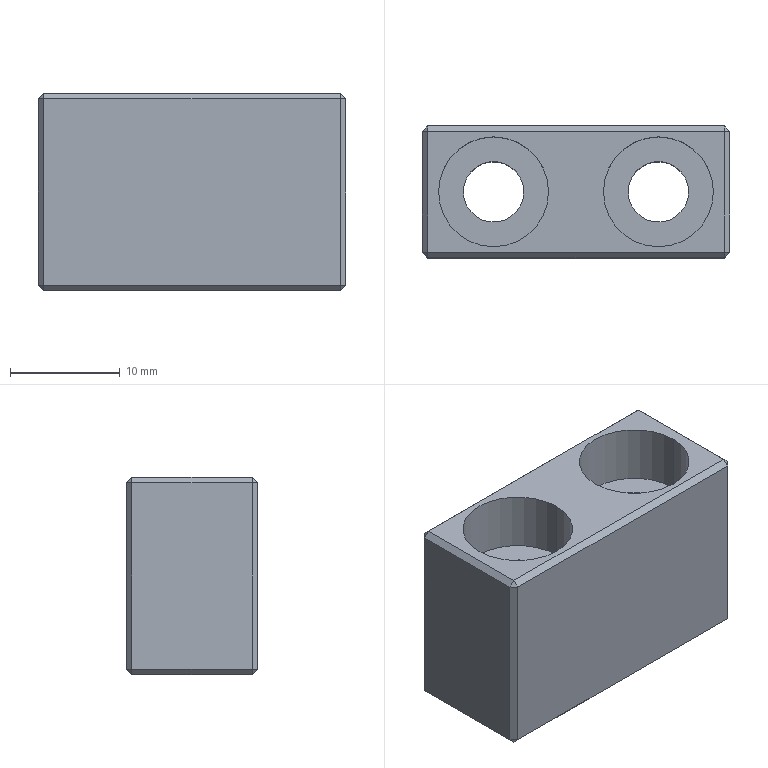Part | SolidWorks | features Chamfer 1, Extrusion 1, HoleWzd 1 | 1 solid | 36 faces | box 28 x 12 x 18 mm | volume 4573 mm3 | plane 28 | cylinder 8 | commonest cylinder face diameters 5.5 x4 10 x4
STEP:
#1=CARTESIAN_POINT('',(-12.5,6.,3.6));
#2=VERTEX_POINT('',#1);
#3=CARTESIAN_POINT('',(-2.5,6.,3.6));
#4=VERTEX_POINT('',#3);
#5=CARTESIAN_POINT('',(-7.5,6.,3.6));
#6=DIRECTION('',(0.,0.,1.));
#7=DIRECTION('',(1.,0.,0.));
#8=AXIS2_PLACEMENT_3D('',#5,#6,#7);
#9=CIRCLE('',#8,5.);
#10=EDGE_CURVE('',#2,#4,#9,.T.);
#11=ORIENTED_EDGE('',*,*,#10,.F.);
#12=CARTESIAN_POINT('',(-12.5,6.,9.));
#13=VERTEX_POINT('',#12);
#14=CARTESIAN_POINT('',(-12.5,6.,9.));
#15=DIRECTION('',(0.,0.,1.));
#16=VECTOR('',#15,1000.);
#17=LINE('',#14,#16);
#18=EDGE_CURVE('',#2,#13,#17,.T.);
#19=ORIENTED_EDGE('',*,*,#18,.T.);
#20=CARTESIAN_POINT('',(-2.5,6.,9.));
#21=VERTEX_POINT('',#20);
#22=CARTESIAN_POINT('',(-7.5,6.,9.));
#23=DIRECTION('',(0.,0.,1.));
#24=DIRECTION('',(1.,0.,0.));
#25=AXIS2_PLACEMENT_3D('',#22,#23,#24);
#26=CIRCLE('',#25,5.);
#27=EDGE_CURVE('',#13,#21,#26,.T.);
#28=ORIENTED_EDGE('',*,*,#27,.T.);
#29=CARTESIAN_POINT('',(-2.5,6.,9.));
#30=DIRECTION('',(0.,0.,1.));
#31=VECTOR('',#30,1000.);
#32=LINE('',#29,#31);
#33=EDGE_CURVE('',#4,#21,#32,.T.);
#34=ORIENTED_EDGE('',*,*,#33,.F.);
#35=EDGE_LOOP('',(#11,#19,#28,#34));
#36=FACE_OUTER_BOUND('',#35,.T.);
#37=CARTESIAN_POINT('',(-7.5,6.,9.));
#38=DIRECTION('',(0.,0.,1.));
#39=DIRECTION('',(1.,0.,0.));
#40=AXIS2_PLACEMENT_3D('',#37,#38,#39);
#41=CYLINDRICAL_SURFACE('',#40,5.);
#42=ADVANCED_FACE('',(#36),#41,.F.);
#43=CARTESIAN_POINT('',(-10.25,6.,-9.));
#44=VERTEX_POINT('',#43);
#45=CARTESIAN_POINT('',(-4.75,6.,-9.));
#46=VERTEX_POINT('',#45);
#47=CARTESIAN_POINT('',(-7.5,6.,-9.));
#48=DIRECTION('',(0.,0.,1.));
#49=DIRECTION('',(1.,0.,0.));
#50=AXIS2_PLACEMENT_3D('',#47,#48,#49);
#51=CIRCLE('',#50,2.75);
#52=EDGE_CURVE('',#44,#46,#51,.T.);
#53=ORIENTED_EDGE('',*,*,#52,.F.);
#54=CARTESIAN_POINT('',(-10.25,6.,3.6));
#55=VERTEX_POINT('',#54);
#56=CARTESIAN_POINT('',(-10.25,6.,9.));
#57=DIRECTION('',(0.,0.,1.));
#58=VECTOR('',#57,1000.);
#59=LINE('',#56,#58);
#60=EDGE_CURVE('',#44,#55,#59,.T.);
#61=ORIENTED_EDGE('',*,*,#60,.T.);
#62=CARTESIAN_POINT('',(-4.75,6.,3.6));
#63=VERTEX_POINT('',#62);
#64=CARTESIAN_POINT('',(-7.5,6.,3.6));
#65=DIRECTION('',(0.,0.,1.));
#66=DIRECTION('',(1.,0.,0.));
#67=AXIS2_PLACEMENT_3D('',#64,#65,#66);
#68=CIRCLE('',#67,2.75);
#69=EDGE_CURVE('',#55,#63,#68,.T.);
#70=ORIENTED_EDGE('',*,*,#69,.T.);
#71=CARTESIAN_POINT('',(-4.75,6.,9.));
#72=DIRECTION('',(0.,0.,1.));
#73=VECTOR('',#72,1000.);
#74=LINE('',#71,#73);
#75=EDGE_CURVE('',#46,#63,#74,.T.);
#76=ORIENTED_EDGE('',*,*,#75,.F.);
#77=EDGE_LOOP('',(#53,#61,#70,#76));
#78=FACE_OUTER_BOUND('',#77,.T.);
#79=CARTESIAN_POINT('',(-7.5,6.,9.));
#80=DIRECTION('',(0.,0.,1.));
#81=DIRECTION('',(1.,0.,0.));
#82=AXIS2_PLACEMENT_3D('',#79,#80,#81);
#83=CYLINDRICAL_SURFACE('',#82,2.75);
#84=ADVANCED_FACE('',(#78),#83,.F.);
#85=CARTESIAN_POINT('',(2.5,6.,3.6));
#86=VERTEX_POINT('',#85);
#87=CARTESIAN_POINT('',(12.5,6.,3.6));
#88=VERTEX_POINT('',#87);
#89=CARTESIAN_POINT('',(7.5,6.,3.6));
#90=DIRECTION('',(0.,0.,1.));
#91=DIRECTION('',(1.,0.,0.));
#92=AXIS2_PLACEMENT_3D('',#89,#90,#91);
#93=CIRCLE('',#92,5.);
#94=EDGE_CURVE('',#86,#88,#93,.T.);
#95=ORIENTED_EDGE('',*,*,#94,.F.);
#96=CARTESIAN_POINT('',(2.5,6.,9.));
#97=VERTEX_POINT('',#96);
#98=CARTESIAN_POINT('',(2.5,6.,9.));
#99=DIRECTION('',(0.,0.,1.));
#100=VECTOR('',#99,1000.);
#101=LINE('',#98,#100);
#102=EDGE_CURVE('',#86,#97,#101,.T.);
#103=ORIENTED_EDGE('',*,*,#102,.T.);
#104=CARTESIAN_POINT('',(12.5,6.,9.));
#105=VERTEX_POINT('',#104);
#106=CARTESIAN_POINT('',(7.5,6.,9.));
#107=DIRECTION('',(0.,0.,1.));
#108=DIRECTION('',(1.,0.,0.));
#109=AXIS2_PLACEMENT_3D('',#106,#107,#108);
#110=CIRCLE('',#109,5.);
#111=EDGE_CURVE('',#97,#105,#110,.T.);
#112=ORIENTED_EDGE('',*,*,#111,.T.);
#113=CARTESIAN_POINT('',(12.5,6.,9.));
#114=DIRECTION('',(0.,0.,1.));
#115=VECTOR('',#114,1000.);
#116=LINE('',#113,#115);
#117=EDGE_CURVE('',#88,#105,#116,.T.);
#118=ORIENTED_EDGE('',*,*,#117,.F.);
#119=EDGE_LOOP('',(#95,#103,#112,#118));
#120=FACE_OUTER_BOUND('',#119,.T.);
#121=CARTESIAN_POINT('',(7.5,6.,9.));
#122=DIRECTION('',(0.,0.,1.));
#123=DIRECTION('',(1.,0.,0.));
#124=AXIS2_PLACEMENT_3D('',#121,#122,#123);
#125=CYLINDRICAL_SURFACE('',#124,5.);
#126=ADVANCED_FACE('',(#120),#125,.F.);
#127=CARTESIAN_POINT('',(4.75,6.,-9.));
#128=VERTEX_POINT('',#127);
#129=CARTESIAN_POINT('',(10.25,6.,-9.));
#130=VERTEX_POINT('',#129);
#131=CARTESIAN_POINT('',(7.5,6.,-9.));
#132=DIRECTION('',(0.,0.,1.));
#133=DIRECTION('',(1.,0.,0.));
#134=AXIS2_PLACEMENT_3D('',#131,#132,#133);
#135=CIRCLE('',#134,2.75);
#136=EDGE_CURVE('',#128,#130,#135,.T.);
#137=ORIENTED_EDGE('',*,*,#136,.F.);
#138=CARTESIAN_POINT('',(4.75,6.,3.6));
#139=VERTEX_POINT('',#138);
#140=CARTESIAN_POINT('',(4.75,6.,9.));
#141=DIRECTION('',(0.,0.,1.));
#142=VECTOR('',#141,1000.);
#143=LINE('',#140,#142);
#144=EDGE_CURVE('',#128,#139,#143,.T.);
#145=ORIENTED_EDGE('',*,*,#144,.T.);
#146=CARTESIAN_POINT('',(10.25,6.,3.6));
#147=VERTEX_POINT('',#146);
#148=CARTESIAN_POINT('',(7.5,6.,3.6));
#149=DIRECTION('',(0.,0.,1.));
#150=DIRECTION('',(1.,0.,0.));
#151=AXIS2_PLACEMENT_3D('',#148,#149,#150);
#152=CIRCLE('',#151,2.75);
#153=EDGE_CURVE('',#139,#147,#152,.T.);
#154=ORIENTED_EDGE('',*,*,#153,.T.);
#155=CARTESIAN_POINT('',(10.25,6.,9.));
#156=DIRECTION('',(0.,0.,1.));
#157=VECTOR('',#156,1000.);
#158=LINE('',#155,#157);
#159=EDGE_CURVE('',#130,#147,#158,.T.);
#160=ORIENTED_EDGE('',*,*,#159,.F.);
#161=EDGE_LOOP('',(#137,#145,#154,#160));
#162=FACE_OUTER_BOUND('',#161,.T.);
#163=CARTESIAN_POINT('',(7.5,6.,9.));
#164=DIRECTION('',(0.,0.,1.));
#165=DIRECTION('',(1.,0.,0.));
#166=AXIS2_PLACEMENT_3D('',#163,#164,#165);
#167=CYLINDRICAL_SURFACE('',#166,2.75);
#168=ADVANCED_FACE('',(#162),#167,.F.);
#169=CARTESIAN_POINT('',(14.,11.5,-8.5));
#170=VERTEX_POINT('',#169);
#171=CARTESIAN_POINT('',(14.,11.5,8.5));
#172=VERTEX_POINT('',#171);
#173=CARTESIAN_POINT('',(14.,11.5,9.));
#174=DIRECTION('',(0.,0.,1.));
#175=VECTOR('',#174,1000.);
#176=LINE('',#173,#175);
#177=EDGE_CURVE('',#170,#172,#176,.T.);
#178=ORIENTED_EDGE('',*,*,#177,.T.);
#179=CARTESIAN_POINT('',(14.,0.5,8.5));
#180=VERTEX_POINT('',#179);
#181=CARTESIAN_POINT('',(14.,12.,8.5));
#182=DIRECTION('',(0.,-1.,0.));
#183=VECTOR('',#182,1000.);
#184=LINE('',#181,#183);
#185=EDGE_CURVE('',#172,#180,#184,.T.);
#186=ORIENTED_EDGE('',*,*,#185,.T.);
#187=CARTESIAN_POINT('',(14.,0.5,-8.5));
#188=VERTEX_POINT('',#187);
#189=CARTESIAN_POINT('',(14.,0.5,-9.));
#190=DIRECTION('',(0.,0.,-1.));
#191=VECTOR('',#190,1000.);
#192=LINE('',#189,#191);
#193=EDGE_CURVE('',#180,#188,#192,.T.);
#194=ORIENTED_EDGE('',*,*,#193,.T.);
#195=CARTESIAN_POINT('',(14.,12.,-8.5));
#196=DIRECTION('',(0.,1.,0.));
#197=VECTOR('',#196,1000.);
#198=LINE('',#195,#197);
#199=EDGE_CURVE('',#188,#170,#198,.T.);
#200=ORIENTED_EDGE('',*,*,#199,.T.);
#201=EDGE_LOOP('',(#178,#186,#194,#200));
#202=FACE_OUTER_BOUND('',#201,.T.);
#203=CARTESIAN_POINT('',(14.,12.,-9.));
#204=DIRECTION('',(-1.,0.,0.));
#205=DIRECTION('',(0.,0.,1.));
#206=AXIS2_PLACEMENT_3D('',#203,#204,#205);
#207=PLANE('',#206);
#208=ADVANCED_FACE('',(#202),#207,.F.);
#209=CARTESIAN_POINT('',(13.5,11.5,-9.));
#210=VERTEX_POINT('',#209);
#211=CARTESIAN_POINT('',(13.5,0.5,-9.));
#212=VERTEX_POINT('',#211);
#213=CARTESIAN_POINT('',(13.5,12.,-9.));
#214=DIRECTION('',(0.,-1.,0.));
#215=VECTOR('',#214,1000.);
#216=LINE('',#213,#215);
#217=EDGE_CURVE('',#210,#212,#216,.T.);
#218=ORIENTED_EDGE('',*,*,#217,.T.);
#219=CARTESIAN_POINT('',(-13.5,0.5,-9.));
#220=VERTEX_POINT('',#219);
#221=CARTESIAN_POINT('',(-14.,0.5,-9.));
#222=DIRECTION('',(-1.,0.,0.));
#223=VECTOR('',#222,1000.);
#224=LINE('',#221,#223);
#225=EDGE_CURVE('',#212,#220,#224,.T.);
#226=ORIENTED_EDGE('',*,*,#225,.T.);
#227=CARTESIAN_POINT('',(-13.5,11.5,-9.));
#228=VERTEX_POINT('',#227);
#229=CARTESIAN_POINT('',(-13.5,12.,-9.));
#230=DIRECTION('',(0.,1.,0.));
#231=VECTOR('',#230,1000.);
#232=LINE('',#229,#231);
#233=EDGE_CURVE('',#220,#228,#232,.T.);
#234=ORIENTED_EDGE('',*,*,#233,.T.);
#235=CARTESIAN_POINT('',(14.,11.5,-9.));
#236=DIRECTION('',(1.,0.,0.));
#237=VECTOR('',#236,1000.);
#238=LINE('',#235,#237);
#239=EDGE_CURVE('',#228,#210,#238,.T.);
#240=ORIENTED_EDGE('',*,*,#239,.T.);
#241=EDGE_LOOP('',(#218,#226,#234,#240));
#242=FACE_OUTER_BOUND('',#241,.T.);
#243=CARTESIAN_POINT('',(-7.5,6.,-9.));
#244=DIRECTION('',(0.,0.,1.));
#245=DIRECTION('',(1.,0.,0.));
#246=AXIS2_PLACEMENT_3D('',#243,#244,#245);
#247=CIRCLE('',#246,2.75);
#248=EDGE_CURVE('',#46,#44,#247,.T.);
#249=ORIENTED_EDGE('',*,*,#248,.T.);
#250=ORIENTED_EDGE('',*,*,#52,.T.);
#251=EDGE_LOOP('',(#249,#250));
#252=FACE_BOUND('',#251,.T.);
#253=CARTESIAN_POINT('',(7.5,6.,-9.));
#254=DIRECTION('',(0.,0.,1.));
#255=DIRECTION('',(1.,0.,0.));
#256=AXIS2_PLACEMENT_3D('',#253,#254,#255);
#257=CIRCLE('',#256,2.75);
#258=EDGE_CURVE('',#130,#128,#257,.T.);
#259=ORIENTED_EDGE('',*,*,#258,.T.);
#260=ORIENTED_EDGE('',*,*,#136,.T.);
#261=EDGE_LOOP('',(#259,#260));
#262=FACE_BOUND('',#261,.T.);
#263=CARTESIAN_POINT('',(-14.,12.,-9.));
#264=DIRECTION('',(0.,0.,1.));
#265=DIRECTION('',(1.,0.,0.));
#266=AXIS2_PLACEMENT_3D('',#263,#264,#265);
#267=PLANE('',#266);
#268=ADVANCED_FACE('',(#242,#252,#262),#267,.F.);
#269=CARTESIAN_POINT('',(-14.,11.5,8.5));
#270=VERTEX_POINT('',#269);
#271=CARTESIAN_POINT('',(-14.,11.5,-8.5));
#272=VERTEX_POINT('',#271);
#273=CARTESIAN_POINT('',(-14.,11.5,-9.));
#274=DIRECTION('',(0.,0.,-1.));
#275=VECTOR('',#274,1000.);
#276=LINE('',#273,#275);
#277=EDGE_CURVE('',#270,#272,#276,.T.);
#278=ORIENTED_EDGE('',*,*,#277,.T.);
#279=CARTESIAN_POINT('',(-14.,0.5,-8.5));
#280=VERTEX_POINT('',#279);
#281=CARTESIAN_POINT('',(-14.,12.,-8.5));
#282=DIRECTION('',(0.,-1.,0.));
#283=VECTOR('',#282,1000.);
#284=LINE('',#281,#283);
#285=EDGE_CURVE('',#272,#280,#284,.T.);
#286=ORIENTED_EDGE('',*,*,#285,.T.);
#287=CARTESIAN_POINT('',(-14.,0.5,8.5));
#288=VERTEX_POINT('',#287);
#289=CARTESIAN_POINT('',(-14.,0.5,-9.));
#290=DIRECTION('',(0.,0.,1.));
#291=VECTOR('',#290,1000.);
#292=LINE('',#289,#291);
#293=EDGE_CURVE('',#280,#288,#292,.T.);
#294=ORIENTED_EDGE('',*,*,#293,.T.);
#295=CARTESIAN_POINT('',(-14.,12.,8.5));
#296=DIRECTION('',(0.,1.,0.));
#297=VECTOR('',#296,1000.);
#298=LINE('',#295,#297);
#299=EDGE_CURVE('',#288,#270,#298,.T.);
#300=ORIENTED_EDGE('',*,*,#299,.T.);
#301=EDGE_LOOP('',(#278,#286,#294,#300));
#302=FACE_OUTER_BOUND('',#301,.T.);
#303=CARTESIAN_POINT('',(-14.,12.,-9.));
#304=DIRECTION('',(1.,0.,0.));
#305=DIRECTION('',(0.,0.,-1.));
#306=AXIS2_PLACEMENT_3D('',#303,#304,#305);
#307=PLANE('',#306);
#308=ADVANCED_FACE('',(#302),#307,.F.);
#309=CARTESIAN_POINT('',(-13.5,11.5,9.));
#310=VERTEX_POINT('',#309);
#311=CARTESIAN_POINT('',(-13.5,0.5,9.));
#312=VERTEX_POINT('',#311);
#313=CARTESIAN_POINT('',(-13.5,12.,9.));
#314=DIRECTION('',(0.,-1.,0.));
#315=VECTOR('',#314,1000.);
#316=LINE('',#313,#315);
#317=EDGE_CURVE('',#310,#312,#316,.T.);
#318=ORIENTED_EDGE('',*,*,#317,.T.);
#319=CARTESIAN_POINT('',(13.5,0.5,9.));
#320=VERTEX_POINT('',#319);
#321=CARTESIAN_POINT('',(-14.,0.5,9.));
#322=DIRECTION('',(1.,0.,0.));
#323=VECTOR('',#322,1000.);
#324=LINE('',#321,#323);
#325=EDGE_CURVE('',#312,#320,#324,.T.);
#326=ORIENTED_EDGE('',*,*,#325,.T.);
#327=CARTESIAN_POINT('',(13.5,11.5,9.));
#328=VERTEX_POINT('',#327);
#329=CARTESIAN_POINT('',(13.5,12.,9.));
#330=DIRECTION('',(0.,1.,0.));
#331=VECTOR('',#330,1000.);
#332=LINE('',#329,#331);
#333=EDGE_CURVE('',#320,#328,#332,.T.);
#334=ORIENTED_EDGE('',*,*,#333,.T.);
#335=CARTESIAN_POINT('',(-14.,11.5,9.));
#336=DIRECTION('',(-1.,0.,0.));
#337=VECTOR('',#336,1000.);
#338=LINE('',#335,#337);
#339=EDGE_CURVE('',#328,#310,#338,.T.);
#340=ORIENTED_EDGE('',*,*,#339,.T.);
#341=EDGE_LOOP('',(#318,#326,#334,#340));
#342=FACE_OUTER_BOUND('',#341,.T.);
#343=CARTESIAN_POINT('',(-7.5,6.,9.));
#344=DIRECTION('',(0.,0.,1.));
#345=DIRECTION('',(1.,0.,0.));
#346=AXIS2_PLACEMENT_3D('',#343,#344,#345);
#347=CIRCLE('',#346,5.);
#348=EDGE_CURVE('',#21,#13,#347,.T.);
#349=ORIENTED_EDGE('',*,*,#348,.F.);
#350=ORIENTED_EDGE('',*,*,#27,.F.);
#351=EDGE_LOOP('',(#349,#350));
#352=FACE_BOUND('',#351,.T.);
#353=CARTESIAN_POINT('',(7.5,6.,9.));
#354=DIRECTION('',(0.,0.,1.));
#355=DIRECTION('',(1.,0.,0.));
#356=AXIS2_PLACEMENT_3D('',#353,#354,#355);
#357=CIRCLE('',#356,5.);
#358=EDGE_CURVE('',#105,#97,#357,.T.);
#359=ORIENTED_EDGE('',*,*,#358,.F.);
#360=ORIENTED_EDGE('',*,*,#111,.F.);
#361=EDGE_LOOP('',(#359,#360));
#362=FACE_BOUND('',#361,.T.);
#363=CARTESIAN_POINT('',(-14.,12.,9.));
#364=DIRECTION('',(0.,0.,-1.));
#365=DIRECTION('',(-1.,0.,0.));
#366=AXIS2_PLACEMENT_3D('',#363,#364,#365);
#367=PLANE('',#366);
#368=ADVANCED_FACE('',(#342,#352,#362),#367,.F.);
#369=CARTESIAN_POINT('',(-13.5,12.,-8.5));
#370=VERTEX_POINT('',#369);
#371=CARTESIAN_POINT('',(-13.5,12.,8.5));
#372=VERTEX_POINT('',#371);
#373=CARTESIAN_POINT('',(-13.5,12.,9.));
#374=DIRECTION('',(0.,0.,1.));
#375=VECTOR('',#374,1000.);
#376=LINE('',#373,#375);
#377=EDGE_CURVE('',#370,#372,#376,.T.);
#378=ORIENTED_EDGE('',*,*,#377,.T.);
#379=CARTESIAN_POINT('',(13.5,12.,8.5));
#380=VERTEX_POINT('',#379);
#381=CARTESIAN_POINT('',(14.,12.,8.5));
#382=DIRECTION('',(1.,0.,0.));
#383=VECTOR('',#382,1000.);
#384=LINE('',#381,#383);
#385=EDGE_CURVE('',#372,#380,#384,.T.);
#386=ORIENTED_EDGE('',*,*,#385,.T.);
#387=CARTESIAN_POINT('',(13.5,12.,-8.5));
#388=VERTEX_POINT('',#387);
#389=CARTESIAN_POINT('',(13.5,12.,-9.));
#390=DIRECTION('',(0.,0.,-1.));
#391=VECTOR('',#390,1000.);
#392=LINE('',#389,#391);
#393=EDGE_CURVE('',#380,#388,#392,.T.);
#394=ORIENTED_EDGE('',*,*,#393,.T.);
#395=CARTESIAN_POINT('',(-14.,12.,-8.5));
#396=DIRECTION('',(-1.,0.,0.));
#397=VECTOR('',#396,1000.);
#398=LINE('',#395,#397);
#399=EDGE_CURVE('',#388,#370,#398,.T.);
#400=ORIENTED_EDGE('',*,*,#399,.T.);
#401=EDGE_LOOP('',(#378,#386,#394,#400));
#402=FACE_OUTER_BOUND('',#401,.T.);
#403=CARTESIAN_POINT('',(0.,12.,0.));
#404=DIRECTION('',(0.,1.,0.));
#405=DIRECTION('',(0.,0.,1.));
#406=AXIS2_PLACEMENT_3D('',#403,#404,#405);
#407=PLANE('',#406);
#408=ADVANCED_FACE('',(#402),#407,.T.);
#409=CARTESIAN_POINT('',(13.5,0.,8.5));
#410=VERTEX_POINT('',#409);
#411=CARTESIAN_POINT('',(-13.5,0.,8.5));
#412=VERTEX_POINT('',#411);
#413=CARTESIAN_POINT('',(0.,0.,8.5));
#414=DIRECTION('',(-1.,0.,0.));
#415=VECTOR('',#414,1000.);
#416=LINE('',#413,#415);
#417=EDGE_CURVE('',#410,#412,#416,.T.);
#418=ORIENTED_EDGE('',*,*,#417,.T.);
#419=CARTESIAN_POINT('',(-13.5,0.,-8.5));
#420=VERTEX_POINT('',#419);
#421=CARTESIAN_POINT('',(-13.5,0.,0.));
#422=DIRECTION('',(0.,0.,-1.));
#423=VECTOR('',#422,1000.);
#424=LINE('',#421,#423);
#425=EDGE_CURVE('',#412,#420,#424,.T.);
#426=ORIENTED_EDGE('',*,*,#425,.T.);
#427=CARTESIAN_POINT('',(13.5,0.,-8.5));
#428=VERTEX_POINT('',#427);
#429=CARTESIAN_POINT('',(0.,0.,-8.5));
#430=DIRECTION('',(1.,0.,0.));
#431=VECTOR('',#430,1000.);
#432=LINE('',#429,#431);
#433=EDGE_CURVE('',#420,#428,#432,.T.);
#434=ORIENTED_EDGE('',*,*,#433,.T.);
#435=CARTESIAN_POINT('',(13.5,0.,0.));
#436=DIRECTION('',(0.,0.,1.));
#437=VECTOR('',#436,1000.);
#438=LINE('',#435,#437);
#439=EDGE_CURVE('',#428,#410,#438,.T.);
#440=ORIENTED_EDGE('',*,*,#439,.T.);
#441=EDGE_LOOP('',(#418,#426,#434,#440));
#442=FACE_OUTER_BOUND('',#441,.T.);
#443=CARTESIAN_POINT('',(0.,0.,0.));
#444=DIRECTION('',(0.,1.,0.));
#445=DIRECTION('',(0.,0.,1.));
#446=AXIS2_PLACEMENT_3D('',#443,#444,#445);
#447=PLANE('',#446);
#448=ADVANCED_FACE('',(#442),#447,.F.);
#449=ORIENTED_EDGE('',*,*,#144,.F.);
#450=ORIENTED_EDGE('',*,*,#258,.F.);
#451=ORIENTED_EDGE('',*,*,#159,.T.);
#452=CARTESIAN_POINT('',(7.5,6.,3.6));
#453=DIRECTION('',(0.,0.,1.));
#454=DIRECTION('',(1.,0.,0.));
#455=AXIS2_PLACEMENT_3D('',#452,#453,#454);
#456=CIRCLE('',#455,2.75);
#457=EDGE_CURVE('',#147,#139,#456,.T.);
#458=ORIENTED_EDGE('',*,*,#457,.T.);
#459=EDGE_LOOP('',(#449,#450,#451,#458));
#460=FACE_OUTER_BOUND('',#459,.T.);
#461=CARTESIAN_POINT('',(7.5,6.,9.));
#462=DIRECTION('',(0.,0.,1.));
#463=DIRECTION('',(1.,0.,0.));
#464=AXIS2_PLACEMENT_3D('',#461,#462,#463);
#465=CYLINDRICAL_SURFACE('',#464,2.75);
#466=ADVANCED_FACE('',(#460),#465,.F.);
#467=ORIENTED_EDGE('',*,*,#457,.F.);
#468=ORIENTED_EDGE('',*,*,#153,.F.);
#469=EDGE_LOOP('',(#467,#468));
#470=FACE_BOUND('',#469,.T.);
#471=CARTESIAN_POINT('',(7.5,6.,3.6));
#472=DIRECTION('',(0.,0.,1.));
#473=DIRECTION('',(1.,0.,0.));
#474=AXIS2_PLACEMENT_3D('',#471,#472,#473);
#475=CIRCLE('',#474,5.);
#476=EDGE_CURVE('',#88,#86,#475,.T.);
#477=ORIENTED_EDGE('',*,*,#476,.T.);
#478=ORIENTED_EDGE('',*,*,#94,.T.);
#479=EDGE_LOOP('',(#477,#478));
#480=FACE_OUTER_BOUND('',#479,.T.);
#481=CARTESIAN_POINT('',(10.25,6.,3.6));
#482=DIRECTION('',(0.,0.,-1.));
#483=DIRECTION('',(-1.,0.,0.));
#484=AXIS2_PLACEMENT_3D('',#481,#482,#483);
#485=PLANE('',#484);
#486=ADVANCED_FACE('',(#470,#480),#485,.F.);
#487=ORIENTED_EDGE('',*,*,#102,.F.);
#488=ORIENTED_EDGE('',*,*,#476,.F.);
#489=ORIENTED_EDGE('',*,*,#117,.T.);
#490=ORIENTED_EDGE('',*,*,#358,.T.);
#491=EDGE_LOOP('',(#487,#488,#489,#490));
#492=FACE_OUTER_BOUND('',#491,.T.);
#493=CARTESIAN_POINT('',(7.5,6.,9.));
#494=DIRECTION('',(0.,0.,1.));
#495=DIRECTION('',(1.,0.,0.));
#496=AXIS2_PLACEMENT_3D('',#493,#494,#495);
#497=CYLINDRICAL_SURFACE('',#496,5.);
#498=ADVANCED_FACE('',(#492),#497,.F.);
#499=ORIENTED_EDGE('',*,*,#60,.F.);
#500=ORIENTED_EDGE('',*,*,#248,.F.);
#501=ORIENTED_EDGE('',*,*,#75,.T.);
#502=CARTESIAN_POINT('',(-7.5,6.,3.6));
#503=DIRECTION('',(0.,0.,1.));
#504=DIRECTION('',(1.,0.,0.));
#505=AXIS2_PLACEMENT_3D('',#502,#503,#504);
#506=CIRCLE('',#505,2.75);
#507=EDGE_CURVE('',#63,#55,#506,.T.);
#508=ORIENTED_EDGE('',*,*,#507,.T.);
#509=EDGE_LOOP('',(#499,#500,#501,#508));
#510=FACE_OUTER_BOUND('',#509,.T.);
#511=CARTESIAN_POINT('',(-7.5,6.,9.));
#512=DIRECTION('',(0.,0.,1.));
#513=DIRECTION('',(1.,0.,0.));
#514=AXIS2_PLACEMENT_3D('',#511,#512,#513);
#515=CYLINDRICAL_SURFACE('',#514,2.75);
#516=ADVANCED_FACE('',(#510),#515,.F.);
#517=ORIENTED_EDGE('',*,*,#507,.F.);
#518=ORIENTED_EDGE('',*,*,#69,.F.);
#519=EDGE_LOOP('',(#517,#518));
#520=FACE_BOUND('',#519,.T.);
#521=CARTESIAN_POINT('',(-7.5,6.,3.6));
#522=DIRECTION('',(0.,0.,1.));
#523=DIRECTION('',(1.,0.,0.));
#524=AXIS2_PLACEMENT_3D('',#521,#522,#523);
#525=CIRCLE('',#524,5.);
#526=EDGE_CURVE('',#4,#2,#525,.T.);
#527=ORIENTED_EDGE('',*,*,#526,.T.);
#528=ORIENTED_EDGE('',*,*,#10,.T.);
#529=EDGE_LOOP('',(#527,#528));
#530=FACE_OUTER_BOUND('',#529,.T.);
#531=CARTESIAN_POINT('',(-4.75,6.,3.6));
#532=DIRECTION('',(0.,0.,-1.));
#533=DIRECTION('',(-1.,0.,0.));
#534=AXIS2_PLACEMENT_3D('',#531,#532,#533);
#535=PLANE('',#534);
#536=ADVANCED_FACE('',(#520,#530),#535,.F.);
#537=ORIENTED_EDGE('',*,*,#18,.F.);
#538=ORIENTED_EDGE('',*,*,#526,.F.);
#539=ORIENTED_EDGE('',*,*,#33,.T.);
#540=ORIENTED_EDGE('',*,*,#348,.T.);
#541=EDGE_LOOP('',(#537,#538,#539,#540));
#542=FACE_OUTER_BOUND('',#541,.T.);
#543=CARTESIAN_POINT('',(-7.5,6.,9.));
#544=DIRECTION('',(0.,0.,1.));
#545=DIRECTION('',(1.,0.,0.));
#546=AXIS2_PLACEMENT_3D('',#543,#544,#545);
#547=CYLINDRICAL_SURFACE('',#546,5.);
#548=ADVANCED_FACE('',(#542),#547,.F.);
#549=CARTESIAN_POINT('',(13.5,12.,8.5));
#550=DIRECTION('',(0.,-0.7071,0.7071));
#551=VECTOR('',#550,1000.);
#552=LINE('',#549,#551);
#553=EDGE_CURVE('',#380,#328,#552,.T.);
#554=ORIENTED_EDGE('',*,*,#553,.F.);
#555=ORIENTED_EDGE('',*,*,#385,.F.);
#556=CARTESIAN_POINT('',(-13.5,11.75,8.75));
#557=DIRECTION('',(0.,0.7071,-0.7071));
#558=VECTOR('',#557,1000.);
#559=LINE('',#556,#558);
#560=EDGE_CURVE('',#310,#372,#559,.T.);
#561=ORIENTED_EDGE('',*,*,#560,.F.);
#562=ORIENTED_EDGE('',*,*,#339,.F.);
#563=EDGE_LOOP('',(#554,#555,#561,#562));
#564=FACE_OUTER_BOUND('',#563,.T.);
#565=CARTESIAN_POINT('',(0.,12.,8.5));
#566=DIRECTION('',(0.,0.7071,0.7071));
#567=DIRECTION('',(-1.,0.,0.));
#568=AXIS2_PLACEMENT_3D('',#565,#566,#567);
#569=PLANE('',#568);
#570=ADVANCED_FACE('',(#564),#569,.T.);
#571=CARTESIAN_POINT('',(13.5,12.,8.5));
#572=DIRECTION('',(0.7071,-0.7071,0.));
#573=VECTOR('',#572,1000.);
#574=LINE('',#571,#573);
#575=EDGE_CURVE('',#380,#172,#574,.T.);
#576=ORIENTED_EDGE('',*,*,#575,.F.);
#577=ORIENTED_EDGE('',*,*,#553,.T.);
#578=CARTESIAN_POINT('',(13.75,11.5,8.75));
#579=DIRECTION('',(-0.7071,0.,0.7071));
#580=VECTOR('',#579,1000.);
#581=LINE('',#578,#580);
#582=EDGE_CURVE('',#172,#328,#581,.T.);
#583=ORIENTED_EDGE('',*,*,#582,.F.);
#584=EDGE_LOOP('',(#576,#577,#583));
#585=FACE_OUTER_BOUND('',#584,.T.);
#586=CARTESIAN_POINT('',(13.5,12.,8.5));
#587=DIRECTION('',(0.5774,0.5774,0.5774));
#588=DIRECTION('',(0.,-0.7071,0.7071));
#589=AXIS2_PLACEMENT_3D('',#586,#587,#588);
#590=PLANE('',#589);
#591=ADVANCED_FACE('',(#585),#590,.T.);
#592=CARTESIAN_POINT('',(-14.,11.5,8.5));
#593=DIRECTION('',(-0.7071,0.,-0.7071));
#594=VECTOR('',#593,1000.);
#595=LINE('',#592,#594);
#596=EDGE_CURVE('',#310,#270,#595,.T.);
#597=ORIENTED_EDGE('',*,*,#596,.F.);
#598=ORIENTED_EDGE('',*,*,#560,.T.);
#599=CARTESIAN_POINT('',(-14.,11.5,8.5));
#600=DIRECTION('',(0.7071,0.7071,0.));
#601=VECTOR('',#600,1000.);
#602=LINE('',#599,#601);
#603=EDGE_CURVE('',#270,#372,#602,.T.);
#604=ORIENTED_EDGE('',*,*,#603,.F.);
#605=EDGE_LOOP('',(#597,#598,#604));
#606=FACE_OUTER_BOUND('',#605,.T.);
#607=CARTESIAN_POINT('',(-14.,11.5,8.5));
#608=DIRECTION('',(-0.5774,0.5774,0.5774));
#609=DIRECTION('',(0.7071,0.,0.7071));
#610=AXIS2_PLACEMENT_3D('',#607,#608,#609);
#611=PLANE('',#610);
#612=ADVANCED_FACE('',(#606),#611,.T.);
#613=ORIENTED_EDGE('',*,*,#582,.T.);
#614=ORIENTED_EDGE('',*,*,#333,.F.);
#615=CARTESIAN_POINT('',(13.5,0.5,9.));
#616=DIRECTION('',(-0.7071,0.,0.7071));
#617=VECTOR('',#616,1000.);
#618=LINE('',#615,#617);
#619=EDGE_CURVE('',#180,#320,#618,.T.);
#620=ORIENTED_EDGE('',*,*,#619,.F.);
#621=ORIENTED_EDGE('',*,*,#185,.F.);
#622=EDGE_LOOP('',(#613,#614,#620,#621));
#623=FACE_OUTER_BOUND('',#622,.T.);
#624=CARTESIAN_POINT('',(14.,12.,8.5));
#625=DIRECTION('',(-0.7071,0.,-0.7071));
#626=DIRECTION('',(0.,-1.,0.));
#627=AXIS2_PLACEMENT_3D('',#624,#625,#626);
#628=PLANE('',#627);
#629=ADVANCED_FACE('',(#623),#628,.F.);
#630=ORIENTED_EDGE('',*,*,#575,.T.);
#631=ORIENTED_EDGE('',*,*,#177,.F.);
#632=CARTESIAN_POINT('',(13.75,11.75,-8.5));
#633=DIRECTION('',(0.7071,-0.7071,0.));
#634=VECTOR('',#633,1000.);
#635=LINE('',#632,#634);
#636=EDGE_CURVE('',#388,#170,#635,.T.);
#637=ORIENTED_EDGE('',*,*,#636,.F.);
#638=ORIENTED_EDGE('',*,*,#393,.F.);
#639=EDGE_LOOP('',(#630,#631,#637,#638));
#640=FACE_OUTER_BOUND('',#639,.T.);
#641=CARTESIAN_POINT('',(13.5,12.,0.));
#642=DIRECTION('',(0.7071,0.7071,0.));
#643=DIRECTION('',(0.,0.,1.));
#644=AXIS2_PLACEMENT_3D('',#641,#642,#643);
#645=PLANE('',#644);
#646=ADVANCED_FACE('',(#640),#645,.T.);
#647=CARTESIAN_POINT('',(-13.5,11.5,-9.));
#648=DIRECTION('',(0.,-0.7071,-0.7071));
#649=VECTOR('',#648,1000.);
#650=LINE('',#647,#649);
#651=EDGE_CURVE('',#370,#228,#650,.T.);
#652=ORIENTED_EDGE('',*,*,#651,.F.);
#653=ORIENTED_EDGE('',*,*,#399,.F.);
#654=CARTESIAN_POINT('',(13.5,11.5,-9.));
#655=DIRECTION('',(0.,0.7071,0.7071));
#656=VECTOR('',#655,1000.);
#657=LINE('',#654,#656);
#658=EDGE_CURVE('',#210,#388,#657,.T.);
#659=ORIENTED_EDGE('',*,*,#658,.F.);
#660=ORIENTED_EDGE('',*,*,#239,.F.);
#661=EDGE_LOOP('',(#652,#653,#659,#660));
#662=FACE_OUTER_BOUND('',#661,.T.);
#663=CARTESIAN_POINT('',(0.,12.,-8.5));
#664=DIRECTION('',(0.,0.7071,-0.7071));
#665=DIRECTION('',(1.,0.,0.));
#666=AXIS2_PLACEMENT_3D('',#663,#664,#665);
#667=PLANE('',#666);
#668=ADVANCED_FACE('',(#662),#667,.T.);
#669=ORIENTED_EDGE('',*,*,#603,.T.);
#670=ORIENTED_EDGE('',*,*,#377,.F.);
#671=CARTESIAN_POINT('',(-13.75,11.75,-8.5));
#672=DIRECTION('',(0.7071,0.7071,0.));
#673=VECTOR('',#672,1000.);
#674=LINE('',#671,#673);
#675=EDGE_CURVE('',#272,#370,#674,.T.);
#676=ORIENTED_EDGE('',*,*,#675,.F.);
#677=ORIENTED_EDGE('',*,*,#277,.F.);
#678=EDGE_LOOP('',(#669,#670,#676,#677));
#679=FACE_OUTER_BOUND('',#678,.T.);
#680=CARTESIAN_POINT('',(-13.5,12.,0.));
#681=DIRECTION('',(-0.7071,0.7071,0.));
#682=DIRECTION('',(0.,0.,-1.));
#683=AXIS2_PLACEMENT_3D('',#680,#681,#682);
#684=PLANE('',#683);
#685=ADVANCED_FACE('',(#679),#684,.T.);
#686=ORIENTED_EDGE('',*,*,#596,.T.);
#687=ORIENTED_EDGE('',*,*,#299,.F.);
#688=CARTESIAN_POINT('',(-13.75,0.5,8.75));
#689=DIRECTION('',(-0.7071,0.,-0.7071));
#690=VECTOR('',#689,1000.);
#691=LINE('',#688,#690);
#692=EDGE_CURVE('',#312,#288,#691,.T.);
#693=ORIENTED_EDGE('',*,*,#692,.F.);
#694=ORIENTED_EDGE('',*,*,#317,.F.);
#695=EDGE_LOOP('',(#686,#687,#693,#694));
#696=FACE_OUTER_BOUND('',#695,.T.);
#697=CARTESIAN_POINT('',(-13.5,12.,9.));
#698=DIRECTION('',(0.7071,0.,-0.7071));
#699=DIRECTION('',(0.,-1.,0.));
#700=AXIS2_PLACEMENT_3D('',#697,#698,#699);
#701=PLANE('',#700);
#702=ADVANCED_FACE('',(#696),#701,.F.);
#703=CARTESIAN_POINT('',(13.5,0.5,9.));
#704=DIRECTION('',(0.,-0.7071,-0.7071));
#705=VECTOR('',#704,1000.);
#706=LINE('',#703,#705);
#707=EDGE_CURVE('',#320,#410,#706,.T.);
#708=ORIENTED_EDGE('',*,*,#707,.F.);
#709=ORIENTED_EDGE('',*,*,#325,.F.);
#710=CARTESIAN_POINT('',(-13.5,0.,8.5));
#711=DIRECTION('',(0.,0.7071,0.7071));
#712=VECTOR('',#711,1000.);
#713=LINE('',#710,#712);
#714=EDGE_CURVE('',#412,#312,#713,.T.);
#715=ORIENTED_EDGE('',*,*,#714,.F.);
#716=ORIENTED_EDGE('',*,*,#417,.F.);
#717=EDGE_LOOP('',(#708,#709,#715,#716));
#718=FACE_OUTER_BOUND('',#717,.T.);
#719=CARTESIAN_POINT('',(-14.,0.5,9.));
#720=DIRECTION('',(0.,0.7071,-0.7071));
#721=DIRECTION('',(1.,0.,0.));
#722=AXIS2_PLACEMENT_3D('',#719,#720,#721);
#723=PLANE('',#722);
#724=ADVANCED_FACE('',(#718),#723,.F.);
#725=ORIENTED_EDGE('',*,*,#619,.T.);
#726=ORIENTED_EDGE('',*,*,#707,.T.);
#727=CARTESIAN_POINT('',(13.75,0.25,8.5));
#728=DIRECTION('',(-0.7071,-0.7071,0.));
#729=VECTOR('',#728,1000.);
#730=LINE('',#727,#729);
#731=EDGE_CURVE('',#180,#410,#730,.T.);
#732=ORIENTED_EDGE('',*,*,#731,.F.);
#733=EDGE_LOOP('',(#725,#726,#732));
#734=FACE_OUTER_BOUND('',#733,.T.);
#735=CARTESIAN_POINT('',(13.5,0.5,9.));
#736=DIRECTION('',(0.5774,-0.5774,0.5774));
#737=DIRECTION('',(0.,-0.7071,-0.7071));
#738=AXIS2_PLACEMENT_3D('',#735,#736,#737);
#739=PLANE('',#738);
#740=ADVANCED_FACE('',(#734),#739,.T.);
#741=ORIENTED_EDGE('',*,*,#658,.T.);
#742=ORIENTED_EDGE('',*,*,#636,.T.);
#743=CARTESIAN_POINT('',(13.5,11.5,-9.));
#744=DIRECTION('',(0.7071,0.,0.7071));
#745=VECTOR('',#744,1000.);
#746=LINE('',#743,#745);
#747=EDGE_CURVE('',#210,#170,#746,.T.);
#748=ORIENTED_EDGE('',*,*,#747,.F.);
#749=EDGE_LOOP('',(#741,#742,#748));
#750=FACE_OUTER_BOUND('',#749,.T.);
#751=CARTESIAN_POINT('',(13.5,11.5,-9.));
#752=DIRECTION('',(0.5774,0.5774,-0.5774));
#753=DIRECTION('',(0.,0.7071,0.7071));
#754=AXIS2_PLACEMENT_3D('',#751,#752,#753);
#755=PLANE('',#754);
#756=ADVANCED_FACE('',(#750),#755,.T.);
#757=ORIENTED_EDGE('',*,*,#675,.T.);
#758=ORIENTED_EDGE('',*,*,#651,.T.);
#759=CARTESIAN_POINT('',(-13.5,11.5,-9.));
#760=DIRECTION('',(0.7071,0.,-0.7071));
#761=VECTOR('',#760,1000.);
#762=LINE('',#759,#761);
#763=EDGE_CURVE('',#272,#228,#762,.T.);
#764=ORIENTED_EDGE('',*,*,#763,.F.);
#765=EDGE_LOOP('',(#757,#758,#764));
#766=FACE_OUTER_BOUND('',#765,.T.);
#767=CARTESIAN_POINT('',(-13.5,11.5,-9.));
#768=DIRECTION('',(-0.5774,0.5774,-0.5774));
#769=DIRECTION('',(-0.7071,0.,0.7071));
#770=AXIS2_PLACEMENT_3D('',#767,#768,#769);
#771=PLANE('',#770);
#772=ADVANCED_FACE('',(#766),#771,.T.);
#773=ORIENTED_EDGE('',*,*,#714,.T.);
#774=ORIENTED_EDGE('',*,*,#692,.T.);
#775=CARTESIAN_POINT('',(-13.5,0.,8.5));
#776=DIRECTION('',(-0.7071,0.7071,0.));
#777=VECTOR('',#776,1000.);
#778=LINE('',#775,#777);
#779=EDGE_CURVE('',#412,#288,#778,.T.);
#780=ORIENTED_EDGE('',*,*,#779,.F.);
#781=EDGE_LOOP('',(#773,#774,#780));
#782=FACE_OUTER_BOUND('',#781,.T.);
#783=CARTESIAN_POINT('',(-13.5,0.,8.5));
#784=DIRECTION('',(-0.5774,-0.5774,0.5774));
#785=DIRECTION('',(0.7071,-0.7071,0.));
#786=AXIS2_PLACEMENT_3D('',#783,#784,#785);
#787=PLANE('',#786);
#788=ADVANCED_FACE('',(#782),#787,.T.);
#789=ORIENTED_EDGE('',*,*,#731,.T.);
#790=ORIENTED_EDGE('',*,*,#439,.F.);
#791=CARTESIAN_POINT('',(13.5,0.,-8.5));
#792=DIRECTION('',(-0.7071,-0.7071,0.));
#793=VECTOR('',#792,1000.);
#794=LINE('',#791,#793);
#795=EDGE_CURVE('',#188,#428,#794,.T.);
#796=ORIENTED_EDGE('',*,*,#795,.F.);
#797=ORIENTED_EDGE('',*,*,#193,.F.);
#798=EDGE_LOOP('',(#789,#790,#796,#797));
#799=FACE_OUTER_BOUND('',#798,.T.);
#800=CARTESIAN_POINT('',(14.,0.5,-9.));
#801=DIRECTION('',(-0.7071,0.7071,0.));
#802=DIRECTION('',(0.,0.,-1.));
#803=AXIS2_PLACEMENT_3D('',#800,#801,#802);
#804=PLANE('',#803);
#805=ADVANCED_FACE('',(#799),#804,.F.);
#806=ORIENTED_EDGE('',*,*,#747,.T.);
#807=ORIENTED_EDGE('',*,*,#199,.F.);
#808=CARTESIAN_POINT('',(13.75,0.5,-8.75));
#809=DIRECTION('',(0.7071,0.,0.7071));
#810=VECTOR('',#809,1000.);
#811=LINE('',#808,#810);
#812=EDGE_CURVE('',#212,#188,#811,.T.);
#813=ORIENTED_EDGE('',*,*,#812,.F.);
#814=ORIENTED_EDGE('',*,*,#217,.F.);
#815=EDGE_LOOP('',(#806,#807,#813,#814));
#816=FACE_OUTER_BOUND('',#815,.T.);
#817=CARTESIAN_POINT('',(13.5,12.,-9.));
#818=DIRECTION('',(-0.7071,0.,0.7071));
#819=DIRECTION('',(0.,-1.,0.));
#820=AXIS2_PLACEMENT_3D('',#817,#818,#819);
#821=PLANE('',#820);
#822=ADVANCED_FACE('',(#816),#821,.F.);
#823=ORIENTED_EDGE('',*,*,#763,.T.);
#824=ORIENTED_EDGE('',*,*,#233,.F.);
#825=CARTESIAN_POINT('',(-13.5,0.5,-9.));
#826=DIRECTION('',(0.7071,0.,-0.7071));
#827=VECTOR('',#826,1000.);
#828=LINE('',#825,#827);
#829=EDGE_CURVE('',#280,#220,#828,.T.);
#830=ORIENTED_EDGE('',*,*,#829,.F.);
#831=ORIENTED_EDGE('',*,*,#285,.F.);
#832=EDGE_LOOP('',(#823,#824,#830,#831));
#833=FACE_OUTER_BOUND('',#832,.T.);
#834=CARTESIAN_POINT('',(-14.,12.,-8.5));
#835=DIRECTION('',(0.7071,0.,0.7071));
#836=DIRECTION('',(0.,-1.,0.));
#837=AXIS2_PLACEMENT_3D('',#834,#835,#836);
#838=PLANE('',#837);
#839=ADVANCED_FACE('',(#833),#838,.F.);
#840=ORIENTED_EDGE('',*,*,#779,.T.);
#841=ORIENTED_EDGE('',*,*,#293,.F.);
#842=CARTESIAN_POINT('',(-13.75,0.25,-8.5));
#843=DIRECTION('',(-0.7071,0.7071,0.));
#844=VECTOR('',#843,1000.);
#845=LINE('',#842,#844);
#846=EDGE_CURVE('',#420,#280,#845,.T.);
#847=ORIENTED_EDGE('',*,*,#846,.F.);
#848=ORIENTED_EDGE('',*,*,#425,.F.);
#849=EDGE_LOOP('',(#840,#841,#847,#848));
#850=FACE_OUTER_BOUND('',#849,.T.);
#851=CARTESIAN_POINT('',(-14.,0.5,-9.));
#852=DIRECTION('',(0.7071,0.7071,0.));
#853=DIRECTION('',(0.,0.,1.));
#854=AXIS2_PLACEMENT_3D('',#851,#852,#853);
#855=PLANE('',#854);
#856=ADVANCED_FACE('',(#850),#855,.F.);
#857=ORIENTED_EDGE('',*,*,#812,.T.);
#858=ORIENTED_EDGE('',*,*,#795,.T.);
#859=CARTESIAN_POINT('',(13.5,0.,-8.5));
#860=DIRECTION('',(0.,-0.7071,0.7071));
#861=VECTOR('',#860,1000.);
#862=LINE('',#859,#861);
#863=EDGE_CURVE('',#212,#428,#862,.T.);
#864=ORIENTED_EDGE('',*,*,#863,.F.);
#865=EDGE_LOOP('',(#857,#858,#864));
#866=FACE_OUTER_BOUND('',#865,.T.);
#867=CARTESIAN_POINT('',(13.5,0.,-8.5));
#868=DIRECTION('',(0.5774,-0.5774,-0.5774));
#869=DIRECTION('',(0.,0.7071,-0.7071));
#870=AXIS2_PLACEMENT_3D('',#867,#868,#869);
#871=PLANE('',#870);
#872=ADVANCED_FACE('',(#866),#871,.T.);
#873=ORIENTED_EDGE('',*,*,#846,.T.);
#874=ORIENTED_EDGE('',*,*,#829,.T.);
#875=CARTESIAN_POINT('',(-13.5,0.5,-9.));
#876=DIRECTION('',(0.,0.7071,-0.7071));
#877=VECTOR('',#876,1000.);
#878=LINE('',#875,#877);
#879=EDGE_CURVE('',#420,#220,#878,.T.);
#880=ORIENTED_EDGE('',*,*,#879,.F.);
#881=EDGE_LOOP('',(#873,#874,#880));
#882=FACE_OUTER_BOUND('',#881,.T.);
#883=CARTESIAN_POINT('',(-13.5,0.5,-9.));
#884=DIRECTION('',(-0.5774,-0.5774,-0.5774));
#885=DIRECTION('',(0.,0.7071,-0.7071));
#886=AXIS2_PLACEMENT_3D('',#883,#884,#885);
#887=PLANE('',#886);
#888=ADVANCED_FACE('',(#882),#887,.T.);
#889=ORIENTED_EDGE('',*,*,#863,.T.);
#890=ORIENTED_EDGE('',*,*,#433,.F.);
#891=ORIENTED_EDGE('',*,*,#879,.T.);
#892=ORIENTED_EDGE('',*,*,#225,.F.);
#893=EDGE_LOOP('',(#889,#890,#891,#892));
#894=FACE_OUTER_BOUND('',#893,.T.);
#895=CARTESIAN_POINT('',(-14.,0.5,-9.));
#896=DIRECTION('',(0.,0.7071,0.7071));
#897=DIRECTION('',(-1.,0.,0.));
#898=AXIS2_PLACEMENT_3D('',#895,#896,#897);
#899=PLANE('',#898);
#900=ADVANCED_FACE('',(#894),#899,.F.);
#901=CLOSED_SHELL('',(#42,#84,#126,#168,#208,#268,#308,#368,#408,#448,#466,#486,#498,#516,#536,#548,#570,#591,#612,#629,#646,#668,#685,#702,#724,#740,#756,#772,#788,#805,#822,#839,#856,#872,#888,#900));
#902=MANIFOLD_SOLID_BREP('',#901);
#903=CARTESIAN_POINT('',(0.,0.,0.));
#904=DIRECTION('',(0.,0.,1.));
#905=DIRECTION('',(1.,0.,0.));
#906=AXIS2_PLACEMENT_3D('',#903,#904,#905);
#907=(LENGTH_UNIT()NAMED_UNIT(*)SI_UNIT(.MILLI.,.METRE.));
#908=UNCERTAINTY_MEASURE_WITH_UNIT(LENGTH_MEASURE(0.00001),#907,'','');
#909=(NAMED_UNIT(*)PLANE_ANGLE_UNIT()SI_UNIT($,.RADIAN.));
#910=(NAMED_UNIT(*)SI_UNIT($,.STERADIAN.)SOLID_ANGLE_UNIT());
#911=(GEOMETRIC_REPRESENTATION_CONTEXT(3)GLOBAL_UNCERTAINTY_ASSIGNED_CONTEXT((#908))GLOBAL_UNIT_ASSIGNED_CONTEXT((#907,#909,#910))REPRESENTATION_CONTEXT('',''));
#912=ADVANCED_BREP_SHAPE_REPRESENTATION('',(#902,#906),#911);